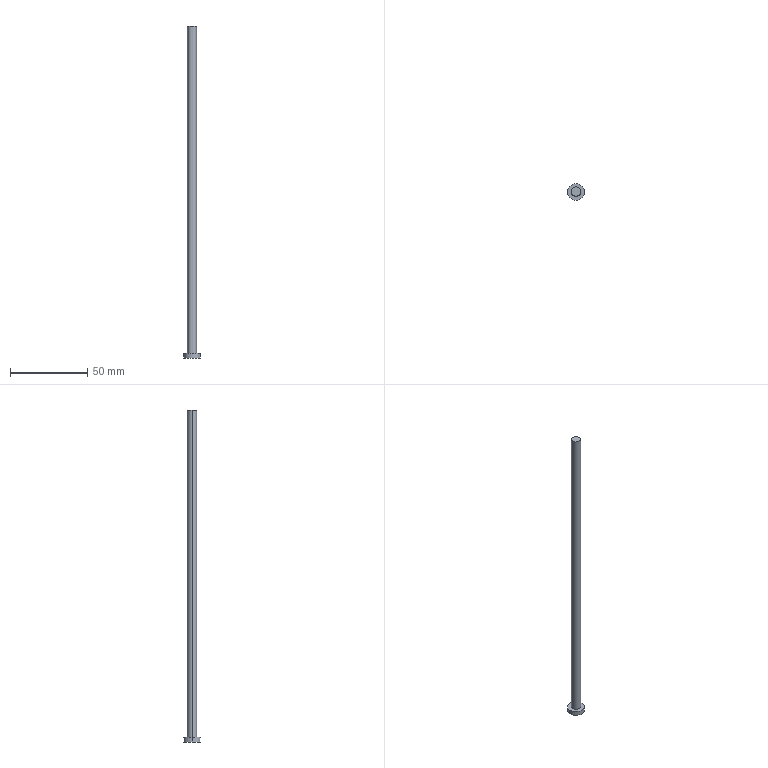Part | Creo | 1 solid | 7 faces | box 11 x 11 x 215 mm | volume 6279 mm3 | cylinder 4 | plane 3 | commonest cylinder face diameters 6 x2 11 x2
STEP:
#1=CARTESIAN_POINT('',(-188.,235.,-232.5));
#2=VERTEX_POINT('',#1);
#3=CARTESIAN_POINT('',(-182.,235.,-232.5));
#4=VERTEX_POINT('',#3);
#5=CARTESIAN_POINT('',(-185.,235.,-232.5));
#6=DIRECTION('',(0.,0.,-1.));
#7=DIRECTION('',(-1.,0.,0.));
#8=AXIS2_PLACEMENT_3D('',#5,#6,#7);
#9=CIRCLE('',#8,3.);
#10=EDGE_CURVE('',#2,#4,#9,.T.);
#11=ORIENTED_EDGE('',*,*,#10,.T.);
#12=CARTESIAN_POINT('',(-182.,235.,-20.5));
#13=VERTEX_POINT('',#12);
#14=CARTESIAN_POINT('',(-182.,235.,-232.5));
#15=DIRECTION('',(0.,0.,1.));
#16=VECTOR('',#15,212.);
#17=LINE('',#14,#16);
#18=EDGE_CURVE('',#4,#13,#17,.T.);
#19=ORIENTED_EDGE('',*,*,#18,.T.);
#20=CARTESIAN_POINT('',(-188.,235.,-20.5));
#21=VERTEX_POINT('',#20);
#22=CARTESIAN_POINT('',(-185.,235.,-20.5));
#23=DIRECTION('',(0.,0.,1.));
#24=DIRECTION('',(1.,0.,0.));
#25=AXIS2_PLACEMENT_3D('',#22,#23,#24);
#26=CIRCLE('',#25,3.);
#27=EDGE_CURVE('',#13,#21,#26,.T.);
#28=ORIENTED_EDGE('',*,*,#27,.T.);
#29=CARTESIAN_POINT('',(-188.,235.,-232.5));
#30=DIRECTION('',(0.,0.,1.));
#31=VECTOR('',#30,212.);
#32=LINE('',#29,#31);
#33=EDGE_CURVE('',#2,#21,#32,.T.);
#34=ORIENTED_EDGE('',*,*,#33,.F.);
#35=EDGE_LOOP('',(#11,#19,#28,#34));
#36=FACE_OUTER_BOUND('',#35,.F.);
#37=CARTESIAN_POINT('',(-185.,235.,-250.296));
#38=DIRECTION('',(0.,0.,1.));
#39=DIRECTION('',(1.,0.,0.));
#40=AXIS2_PLACEMENT_3D('',#37,#38,#39);
#41=CYLINDRICAL_SURFACE('',#40,3.);
#42=ADVANCED_FACE('',(#36),#41,.T.);
#43=CARTESIAN_POINT('',(-179.5,235.,-232.5));
#44=VERTEX_POINT('',#43);
#45=CARTESIAN_POINT('',(-190.5,235.,-232.5));
#46=VERTEX_POINT('',#45);
#47=CARTESIAN_POINT('',(-185.,235.,-232.5));
#48=DIRECTION('',(0.,0.,1.));
#49=DIRECTION('',(1.,0.,0.));
#50=AXIS2_PLACEMENT_3D('',#47,#48,#49);
#51=CIRCLE('',#50,5.5);
#52=EDGE_CURVE('',#44,#46,#51,.T.);
#53=ORIENTED_EDGE('',*,*,#52,.F.);
#54=CARTESIAN_POINT('',(-185.,235.,-232.5));
#55=DIRECTION('',(0.,0.,1.));
#56=DIRECTION('',(-1.,0.,0.));
#57=AXIS2_PLACEMENT_3D('',#54,#55,#56);
#58=CIRCLE('',#57,5.5);
#59=EDGE_CURVE('',#46,#44,#58,.T.);
#60=ORIENTED_EDGE('',*,*,#59,.F.);
#61=EDGE_LOOP('',(#53,#60));
#62=FACE_OUTER_BOUND('',#61,.F.);
#63=CARTESIAN_POINT('',(-185.,235.,-232.5));
#64=DIRECTION('',(0.,0.,-1.));
#65=DIRECTION('',(1.,0.,0.));
#66=AXIS2_PLACEMENT_3D('',#63,#64,#65);
#67=CIRCLE('',#66,3.);
#68=EDGE_CURVE('',#4,#2,#67,.T.);
#69=ORIENTED_EDGE('',*,*,#68,.F.);
#70=ORIENTED_EDGE('',*,*,#10,.F.);
#71=EDGE_LOOP('',(#69,#70));
#72=FACE_BOUND('',#71,.F.);
#73=CARTESIAN_POINT('',(-185.,235.,-232.5));
#74=DIRECTION('',(0.,0.,1.));
#75=DIRECTION('',(1.,0.,0.));
#76=AXIS2_PLACEMENT_3D('',#73,#74,#75);
#77=PLANE('',#76);
#78=ADVANCED_FACE('',(#62,#72),#77,.T.);
#79=CARTESIAN_POINT('',(-190.5,235.,-235.5));
#80=VERTEX_POINT('',#79);
#81=CARTESIAN_POINT('',(-179.5,235.,-235.5));
#82=VERTEX_POINT('',#81);
#83=CARTESIAN_POINT('',(-185.,235.,-235.5));
#84=DIRECTION('',(0.,0.,-1.));
#85=DIRECTION('',(-1.,0.,0.));
#86=AXIS2_PLACEMENT_3D('',#83,#84,#85);
#87=CIRCLE('',#86,5.5);
#88=EDGE_CURVE('',#80,#82,#87,.T.);
#89=ORIENTED_EDGE('',*,*,#88,.T.);
#90=CARTESIAN_POINT('',(-179.5,235.,-235.5));
#91=DIRECTION('',(0.,0.,1.));
#92=VECTOR('',#91,3.);
#93=LINE('',#90,#92);
#94=EDGE_CURVE('',#82,#44,#93,.T.);
#95=ORIENTED_EDGE('',*,*,#94,.T.);
#96=ORIENTED_EDGE('',*,*,#52,.T.);
#97=CARTESIAN_POINT('',(-190.5,235.,-235.5));
#98=DIRECTION('',(0.,0.,1.));
#99=VECTOR('',#98,3.);
#100=LINE('',#97,#99);
#101=EDGE_CURVE('',#80,#46,#100,.T.);
#102=ORIENTED_EDGE('',*,*,#101,.F.);
#103=EDGE_LOOP('',(#89,#95,#96,#102));
#104=FACE_OUTER_BOUND('',#103,.F.);
#105=CARTESIAN_POINT('',(-185.,235.,-241.77));
#106=DIRECTION('',(0.,0.,1.));
#107=DIRECTION('',(1.,0.,0.));
#108=AXIS2_PLACEMENT_3D('',#105,#106,#107);
#109=CYLINDRICAL_SURFACE('',#108,5.5);
#110=ADVANCED_FACE('',(#104),#109,.T.);
#111=CARTESIAN_POINT('',(-185.,235.,-235.5));
#112=DIRECTION('',(0.,0.,-1.));
#113=DIRECTION('',(1.,0.,0.));
#114=AXIS2_PLACEMENT_3D('',#111,#112,#113);
#115=CIRCLE('',#114,5.5);
#116=EDGE_CURVE('',#82,#80,#115,.T.);
#117=ORIENTED_EDGE('',*,*,#116,.F.);
#118=ORIENTED_EDGE('',*,*,#88,.F.);
#119=EDGE_LOOP('',(#117,#118));
#120=FACE_OUTER_BOUND('',#119,.F.);
#121=CARTESIAN_POINT('',(-185.,235.,-235.5));
#122=DIRECTION('',(0.,0.,1.));
#123=DIRECTION('',(1.,0.,0.));
#124=AXIS2_PLACEMENT_3D('',#121,#122,#123);
#125=PLANE('',#124);
#126=ADVANCED_FACE('',(#120),#125,.F.);
#127=ORIENTED_EDGE('',*,*,#116,.T.);
#128=ORIENTED_EDGE('',*,*,#101,.T.);
#129=ORIENTED_EDGE('',*,*,#59,.T.);
#130=ORIENTED_EDGE('',*,*,#94,.F.);
#131=EDGE_LOOP('',(#127,#128,#129,#130));
#132=FACE_OUTER_BOUND('',#131,.F.);
#133=CARTESIAN_POINT('',(-185.,235.,-241.77));
#134=DIRECTION('',(0.,0.,1.));
#135=DIRECTION('',(1.,0.,0.));
#136=AXIS2_PLACEMENT_3D('',#133,#134,#135);
#137=CYLINDRICAL_SURFACE('',#136,5.5);
#138=ADVANCED_FACE('',(#132),#137,.T.);
#139=ORIENTED_EDGE('',*,*,#68,.T.);
#140=ORIENTED_EDGE('',*,*,#33,.T.);
#141=CARTESIAN_POINT('',(-185.,235.,-20.5));
#142=DIRECTION('',(0.,0.,1.));
#143=DIRECTION('',(-1.,0.,0.));
#144=AXIS2_PLACEMENT_3D('',#141,#142,#143);
#145=CIRCLE('',#144,3.);
#146=EDGE_CURVE('',#21,#13,#145,.T.);
#147=ORIENTED_EDGE('',*,*,#146,.T.);
#148=ORIENTED_EDGE('',*,*,#18,.F.);
#149=EDGE_LOOP('',(#139,#140,#147,#148));
#150=FACE_OUTER_BOUND('',#149,.F.);
#151=CARTESIAN_POINT('',(-185.,235.,-250.296));
#152=DIRECTION('',(0.,0.,1.));
#153=DIRECTION('',(1.,0.,0.));
#154=AXIS2_PLACEMENT_3D('',#151,#152,#153);
#155=CYLINDRICAL_SURFACE('',#154,3.);
#156=ADVANCED_FACE('',(#150),#155,.T.);
#157=ORIENTED_EDGE('',*,*,#146,.F.);
#158=ORIENTED_EDGE('',*,*,#27,.F.);
#159=EDGE_LOOP('',(#157,#158));
#160=FACE_OUTER_BOUND('',#159,.F.);
#161=CARTESIAN_POINT('',(-180.5,235.,-20.5));
#162=DIRECTION('',(0.,0.,-1.));
#163=DIRECTION('',(-1.,0.,0.));
#164=AXIS2_PLACEMENT_3D('',#161,#162,#163);
#165=PLANE('',#164);
#166=ADVANCED_FACE('',(#160),#165,.F.);
#167=CLOSED_SHELL('',(#42,#78,#110,#126,#138,#156,#166));
#168=MANIFOLD_SOLID_BREP('',#167);
#169=(LENGTH_UNIT()NAMED_UNIT(*)SI_UNIT(.MILLI.,.METRE.));
#170=UNCERTAINTY_MEASURE_WITH_UNIT(LENGTH_MEASURE(0.02156),#169,'','');
#171=(NAMED_UNIT(*)PLANE_ANGLE_UNIT()SI_UNIT($,.RADIAN.));
#172=PLANE_ANGLE_MEASURE_WITH_UNIT(PLANE_ANGLE_MEASURE(0.01745),#171);
#173=(CONVERSION_BASED_UNIT('DEGREE',#172)NAMED_UNIT(*)PLANE_ANGLE_UNIT());
#174=(NAMED_UNIT(*)SI_UNIT($,.STERADIAN.)SOLID_ANGLE_UNIT());
#175=(GEOMETRIC_REPRESENTATION_CONTEXT(3)GLOBAL_UNCERTAINTY_ASSIGNED_CONTEXT((#170))GLOBAL_UNIT_ASSIGNED_CONTEXT((#169,#173,#174))REPRESENTATION_CONTEXT('',''));
#176=ADVANCED_BREP_SHAPE_REPRESENTATION('',(#168),#175);